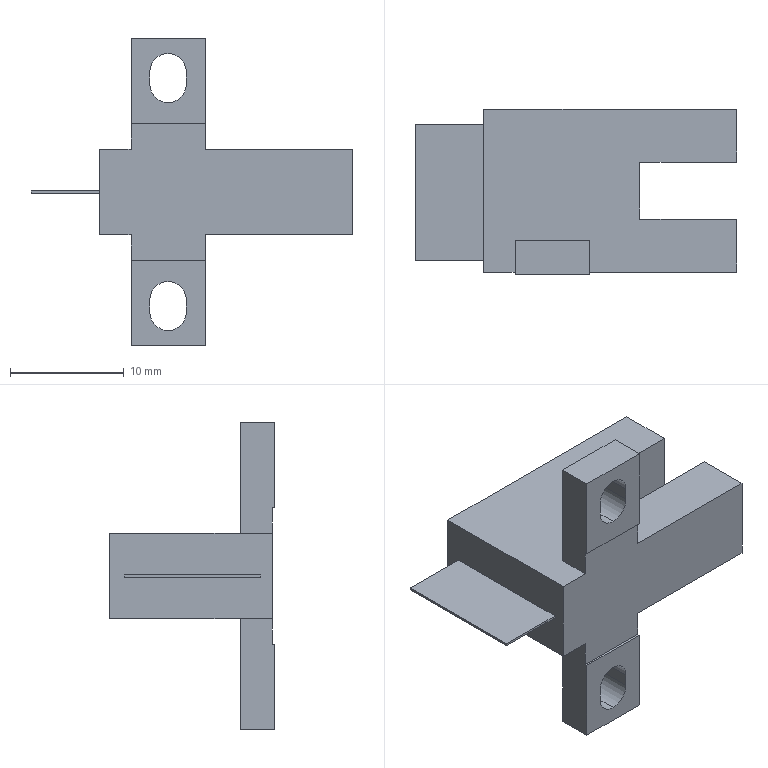Part | SolidWorks | features BaseBody 1 | 1 solid | 37 faces | box 28.2 x 14.5 x 27 mm | volume 2382 mm3 | plane 31 | cylinder 6 | commonest cylinder face diameters 3.2 x6
STEP:
#1=CARTESIAN_POINT('',(6.,2.8,7.85));
#2=VERTEX_POINT('',#1);
#3=CARTESIAN_POINT('',(7.6,2.8,9.45));
#4=VERTEX_POINT('',#3);
#5=CARTESIAN_POINT('',(6.,2.8,9.45));
#6=DIRECTION('',(0.,-1.,0.));
#7=DIRECTION('',(0.,0.,1.));
#8=AXIS2_PLACEMENT_3D('',#5,#6,#7);
#9=CIRCLE('',#8,1.6);
#10=EDGE_CURVE('',#2,#4,#9,.T.);
#11=ORIENTED_EDGE('',*,*,#10,.F.);
#12=CARTESIAN_POINT('',(6.,-0.2,7.85));
#13=VERTEX_POINT('',#12);
#14=CARTESIAN_POINT('',(6.,2.8,7.85));
#15=DIRECTION('',(0.,-1.,0.));
#16=VECTOR('',#15,1000.);
#17=LINE('',#14,#16);
#18=EDGE_CURVE('',#2,#13,#17,.T.);
#19=ORIENTED_EDGE('',*,*,#18,.T.);
#20=CARTESIAN_POINT('',(7.6,-0.2,9.45));
#21=VERTEX_POINT('',#20);
#22=CARTESIAN_POINT('',(6.,-0.2,9.45));
#23=DIRECTION('',(0.,-1.,0.));
#24=DIRECTION('',(0.,0.,1.));
#25=AXIS2_PLACEMENT_3D('',#22,#23,#24);
#26=CIRCLE('',#25,1.6);
#27=EDGE_CURVE('',#13,#21,#26,.T.);
#28=ORIENTED_EDGE('',*,*,#27,.T.);
#29=CARTESIAN_POINT('',(7.6,2.8,9.45));
#30=DIRECTION('',(0.,-1.,0.));
#31=VECTOR('',#30,1000.);
#32=LINE('',#29,#31);
#33=EDGE_CURVE('',#4,#21,#32,.T.);
#34=ORIENTED_EDGE('',*,*,#33,.F.);
#35=EDGE_LOOP('',(#11,#19,#28,#34));
#36=FACE_OUTER_BOUND('',#35,.T.);
#37=CARTESIAN_POINT('',(6.,2.8,9.45));
#38=DIRECTION('',(0.,-1.,0.));
#39=DIRECTION('',(0.,0.,-1.));
#40=AXIS2_PLACEMENT_3D('',#37,#38,#39);
#41=CYLINDRICAL_SURFACE('',#40,1.6);
#42=ADVANCED_FACE('',(#36),#41,.F.);
#43=CARTESIAN_POINT('',(6.,2.8,-12.15));
#44=VERTEX_POINT('',#43);
#45=CARTESIAN_POINT('',(7.6,2.8,-10.55));
#46=VERTEX_POINT('',#45);
#47=CARTESIAN_POINT('',(6.,2.8,-10.55));
#48=DIRECTION('',(0.,-1.,0.));
#49=DIRECTION('',(0.,0.,-1.));
#50=AXIS2_PLACEMENT_3D('',#47,#48,#49);
#51=CIRCLE('',#50,1.6);
#52=EDGE_CURVE('',#44,#46,#51,.T.);
#53=ORIENTED_EDGE('',*,*,#52,.F.);
#54=CARTESIAN_POINT('',(6.,-0.2,-12.15));
#55=VERTEX_POINT('',#54);
#56=CARTESIAN_POINT('',(6.,2.8,-12.15));
#57=DIRECTION('',(0.,-1.,0.));
#58=VECTOR('',#57,1000.);
#59=LINE('',#56,#58);
#60=EDGE_CURVE('',#44,#55,#59,.T.);
#61=ORIENTED_EDGE('',*,*,#60,.T.);
#62=CARTESIAN_POINT('',(7.6,-0.2,-10.55));
#63=VERTEX_POINT('',#62);
#64=CARTESIAN_POINT('',(6.,-0.2,-10.55));
#65=DIRECTION('',(0.,-1.,0.));
#66=DIRECTION('',(0.,0.,-1.));
#67=AXIS2_PLACEMENT_3D('',#64,#65,#66);
#68=CIRCLE('',#67,1.6);
#69=EDGE_CURVE('',#55,#63,#68,.T.);
#70=ORIENTED_EDGE('',*,*,#69,.T.);
#71=CARTESIAN_POINT('',(7.6,2.8,-10.55));
#72=DIRECTION('',(0.,-1.,0.));
#73=VECTOR('',#72,1000.);
#74=LINE('',#71,#73);
#75=EDGE_CURVE('',#46,#63,#74,.T.);
#76=ORIENTED_EDGE('',*,*,#75,.F.);
#77=EDGE_LOOP('',(#53,#61,#70,#76));
#78=FACE_OUTER_BOUND('',#77,.T.);
#79=CARTESIAN_POINT('',(6.,2.8,-10.55));
#80=DIRECTION('',(0.,-1.,0.));
#81=DIRECTION('',(0.,0.,-1.));
#82=AXIS2_PLACEMENT_3D('',#79,#80,#81);
#83=CYLINDRICAL_SURFACE('',#82,1.6);
#84=ADVANCED_FACE('',(#78),#83,.F.);
#85=CARTESIAN_POINT('',(-6.,13.,-0.1));
#86=VERTEX_POINT('',#85);
#87=CARTESIAN_POINT('',(-6.,1.,-0.1));
#88=VERTEX_POINT('',#87);
#89=CARTESIAN_POINT('',(-6.,13.,-0.1));
#90=DIRECTION('',(0.,-1.,0.));
#91=VECTOR('',#90,1000.);
#92=LINE('',#89,#91);
#93=EDGE_CURVE('',#86,#88,#92,.T.);
#94=ORIENTED_EDGE('',*,*,#93,.T.);
#95=CARTESIAN_POINT('',(-6.,1.,0.1));
#96=VERTEX_POINT('',#95);
#97=CARTESIAN_POINT('',(-6.,1.,-0.1));
#98=DIRECTION('',(0.,0.,1.));
#99=VECTOR('',#98,1000.);
#100=LINE('',#97,#99);
#101=EDGE_CURVE('',#88,#96,#100,.T.);
#102=ORIENTED_EDGE('',*,*,#101,.T.);
#103=CARTESIAN_POINT('',(-6.,13.,0.1));
#104=VERTEX_POINT('',#103);
#105=CARTESIAN_POINT('',(-6.,13.,0.1));
#106=DIRECTION('',(0.,1.,0.));
#107=VECTOR('',#106,1000.);
#108=LINE('',#105,#107);
#109=EDGE_CURVE('',#96,#104,#108,.T.);
#110=ORIENTED_EDGE('',*,*,#109,.T.);
#111=CARTESIAN_POINT('',(-6.,13.,-0.1));
#112=DIRECTION('',(0.,0.,-1.));
#113=VECTOR('',#112,1000.);
#114=LINE('',#111,#113);
#115=EDGE_CURVE('',#104,#86,#114,.T.);
#116=ORIENTED_EDGE('',*,*,#115,.T.);
#117=EDGE_LOOP('',(#94,#102,#110,#116));
#118=FACE_OUTER_BOUND('',#117,.T.);
#119=CARTESIAN_POINT('',(-6.,0.,0.));
#120=DIRECTION('',(-1.,0.,0.));
#121=DIRECTION('',(0.,0.,1.));
#122=AXIS2_PLACEMENT_3D('',#119,#120,#121);
#123=PLANE('',#122);
#124=ADVANCED_FACE('',(#118),#123,.T.);
#125=CARTESIAN_POINT('',(0.,13.,0.1));
#126=VERTEX_POINT('',#125);
#127=CARTESIAN_POINT('',(0.,13.,-0.1));
#128=VERTEX_POINT('',#127);
#129=CARTESIAN_POINT('',(0.,13.,-0.1));
#130=DIRECTION('',(0.,0.,-1.));
#131=VECTOR('',#130,1000.);
#132=LINE('',#129,#131);
#133=EDGE_CURVE('',#126,#128,#132,.T.);
#134=ORIENTED_EDGE('',*,*,#133,.T.);
#135=CARTESIAN_POINT('',(-6.,13.,-0.1));
#136=DIRECTION('',(1.,0.,0.));
#137=VECTOR('',#136,1000.);
#138=LINE('',#135,#137);
#139=EDGE_CURVE('',#86,#128,#138,.T.);
#140=ORIENTED_EDGE('',*,*,#139,.F.);
#141=ORIENTED_EDGE('',*,*,#115,.F.);
#142=CARTESIAN_POINT('',(-6.,13.,0.1));
#143=DIRECTION('',(1.,0.,0.));
#144=VECTOR('',#143,1000.);
#145=LINE('',#142,#144);
#146=EDGE_CURVE('',#104,#126,#145,.T.);
#147=ORIENTED_EDGE('',*,*,#146,.T.);
#148=EDGE_LOOP('',(#134,#140,#141,#147));
#149=FACE_OUTER_BOUND('',#148,.T.);
#150=CARTESIAN_POINT('',(-6.,13.,-0.1));
#151=DIRECTION('',(0.,-1.,0.));
#152=DIRECTION('',(-1.,0.,0.));
#153=AXIS2_PLACEMENT_3D('',#150,#151,#152);
#154=PLANE('',#153);
#155=ADVANCED_FACE('',(#149),#154,.F.);
#156=CARTESIAN_POINT('',(0.,1.,0.1));
#157=VERTEX_POINT('',#156);
#158=CARTESIAN_POINT('',(0.,13.,0.1));
#159=DIRECTION('',(0.,1.,0.));
#160=VECTOR('',#159,1000.);
#161=LINE('',#158,#160);
#162=EDGE_CURVE('',#157,#126,#161,.T.);
#163=ORIENTED_EDGE('',*,*,#162,.T.);
#164=ORIENTED_EDGE('',*,*,#146,.F.);
#165=ORIENTED_EDGE('',*,*,#109,.F.);
#166=CARTESIAN_POINT('',(-6.,1.,0.1));
#167=DIRECTION('',(1.,0.,0.));
#168=VECTOR('',#167,1000.);
#169=LINE('',#166,#168);
#170=EDGE_CURVE('',#96,#157,#169,.T.);
#171=ORIENTED_EDGE('',*,*,#170,.T.);
#172=EDGE_LOOP('',(#163,#164,#165,#171));
#173=FACE_OUTER_BOUND('',#172,.T.);
#174=CARTESIAN_POINT('',(-6.,13.,0.1));
#175=DIRECTION('',(0.,0.,-1.));
#176=DIRECTION('',(0.,-1.,0.));
#177=AXIS2_PLACEMENT_3D('',#174,#175,#176);
#178=PLANE('',#177);
#179=ADVANCED_FACE('',(#173),#178,.F.);
#180=CARTESIAN_POINT('',(0.,1.,-0.1));
#181=VERTEX_POINT('',#180);
#182=CARTESIAN_POINT('',(0.,1.,-0.1));
#183=DIRECTION('',(0.,0.,1.));
#184=VECTOR('',#183,1000.);
#185=LINE('',#182,#184);
#186=EDGE_CURVE('',#181,#157,#185,.T.);
#187=ORIENTED_EDGE('',*,*,#186,.T.);
#188=ORIENTED_EDGE('',*,*,#170,.F.);
#189=ORIENTED_EDGE('',*,*,#101,.F.);
#190=CARTESIAN_POINT('',(-6.,1.,-0.1));
#191=DIRECTION('',(1.,0.,0.));
#192=VECTOR('',#191,1000.);
#193=LINE('',#190,#192);
#194=EDGE_CURVE('',#88,#181,#193,.T.);
#195=ORIENTED_EDGE('',*,*,#194,.T.);
#196=EDGE_LOOP('',(#187,#188,#189,#195));
#197=FACE_OUTER_BOUND('',#196,.T.);
#198=CARTESIAN_POINT('',(-6.,1.,-0.1));
#199=DIRECTION('',(0.,1.,0.));
#200=DIRECTION('',(1.,0.,0.));
#201=AXIS2_PLACEMENT_3D('',#198,#199,#200);
#202=PLANE('',#201);
#203=ADVANCED_FACE('',(#197),#202,.F.);
#204=CARTESIAN_POINT('',(0.,13.,-0.1));
#205=DIRECTION('',(0.,-1.,0.));
#206=VECTOR('',#205,1000.);
#207=LINE('',#204,#206);
#208=EDGE_CURVE('',#128,#181,#207,.T.);
#209=ORIENTED_EDGE('',*,*,#208,.T.);
#210=ORIENTED_EDGE('',*,*,#194,.F.);
#211=ORIENTED_EDGE('',*,*,#93,.F.);
#212=ORIENTED_EDGE('',*,*,#139,.T.);
#213=EDGE_LOOP('',(#209,#210,#211,#212));
#214=FACE_OUTER_BOUND('',#213,.T.);
#215=CARTESIAN_POINT('',(-6.,13.,-0.1));
#216=DIRECTION('',(0.,0.,1.));
#217=DIRECTION('',(0.,-1.,0.));
#218=AXIS2_PLACEMENT_3D('',#215,#216,#217);
#219=PLANE('',#218);
#220=ADVANCED_FACE('',(#214),#219,.F.);
#221=CARTESIAN_POINT('',(9.25,-0.2,-6.));
#222=VERTEX_POINT('',#221);
#223=CARTESIAN_POINT('',(9.25,0.,-6.));
#224=VERTEX_POINT('',#223);
#225=CARTESIAN_POINT('',(9.25,-0.201,-6.));
#226=DIRECTION('',(0.,1.,0.));
#227=VECTOR('',#226,1000.);
#228=LINE('',#225,#227);
#229=EDGE_CURVE('',#222,#224,#228,.T.);
#230=ORIENTED_EDGE('',*,*,#229,.T.);
#231=CARTESIAN_POINT('',(2.75,0.,-6.));
#232=VERTEX_POINT('',#231);
#233=CARTESIAN_POINT('',(2.75,0.,-6.));
#234=DIRECTION('',(1.,0.,0.));
#235=VECTOR('',#234,1000.);
#236=LINE('',#233,#235);
#237=EDGE_CURVE('',#232,#224,#236,.T.);
#238=ORIENTED_EDGE('',*,*,#237,.F.);
#239=CARTESIAN_POINT('',(2.75,-0.2,-6.));
#240=VERTEX_POINT('',#239);
#241=CARTESIAN_POINT('',(2.75,-0.201,-6.));
#242=DIRECTION('',(0.,1.,0.));
#243=VECTOR('',#242,1000.);
#244=LINE('',#241,#243);
#245=EDGE_CURVE('',#240,#232,#244,.T.);
#246=ORIENTED_EDGE('',*,*,#245,.F.);
#247=CARTESIAN_POINT('',(2.75,-0.2,-6.));
#248=DIRECTION('',(-1.,0.,0.));
#249=VECTOR('',#248,1000.);
#250=LINE('',#247,#249);
#251=EDGE_CURVE('',#222,#240,#250,.T.);
#252=ORIENTED_EDGE('',*,*,#251,.F.);
#253=EDGE_LOOP('',(#230,#238,#246,#252));
#254=FACE_OUTER_BOUND('',#253,.T.);
#255=CARTESIAN_POINT('',(2.75,-0.201,-6.));
#256=DIRECTION('',(0.,0.,1.));
#257=DIRECTION('',(1.,0.,0.));
#258=AXIS2_PLACEMENT_3D('',#255,#256,#257);
#259=PLANE('',#258);
#260=ADVANCED_FACE('',(#254),#259,.T.);
#261=CARTESIAN_POINT('',(9.25,-0.2,6.));
#262=VERTEX_POINT('',#261);
#263=CARTESIAN_POINT('',(2.75,-0.2,6.));
#264=VERTEX_POINT('',#263);
#265=CARTESIAN_POINT('',(2.75,-0.2,6.));
#266=DIRECTION('',(-1.,0.,0.));
#267=VECTOR('',#266,1000.);
#268=LINE('',#265,#267);
#269=EDGE_CURVE('',#262,#264,#268,.T.);
#270=ORIENTED_EDGE('',*,*,#269,.T.);
#271=CARTESIAN_POINT('',(2.75,0.,6.));
#272=VERTEX_POINT('',#271);
#273=CARTESIAN_POINT('',(2.75,-0.201,6.));
#274=DIRECTION('',(0.,1.,0.));
#275=VECTOR('',#274,1000.);
#276=LINE('',#273,#275);
#277=EDGE_CURVE('',#264,#272,#276,.T.);
#278=ORIENTED_EDGE('',*,*,#277,.T.);
#279=CARTESIAN_POINT('',(9.25,0.,6.));
#280=VERTEX_POINT('',#279);
#281=CARTESIAN_POINT('',(2.75,0.,6.));
#282=DIRECTION('',(-1.,0.,0.));
#283=VECTOR('',#282,1000.);
#284=LINE('',#281,#283);
#285=EDGE_CURVE('',#280,#272,#284,.T.);
#286=ORIENTED_EDGE('',*,*,#285,.F.);
#287=CARTESIAN_POINT('',(9.25,-0.201,6.));
#288=DIRECTION('',(0.,1.,0.));
#289=VECTOR('',#288,1000.);
#290=LINE('',#287,#289);
#291=EDGE_CURVE('',#262,#280,#290,.T.);
#292=ORIENTED_EDGE('',*,*,#291,.F.);
#293=EDGE_LOOP('',(#270,#278,#286,#292));
#294=FACE_OUTER_BOUND('',#293,.T.);
#295=CARTESIAN_POINT('',(2.75,-0.201,6.));
#296=DIRECTION('',(0.,0.,-1.));
#297=DIRECTION('',(0.,-1.,0.));
#298=AXIS2_PLACEMENT_3D('',#295,#296,#297);
#299=PLANE('',#298);
#300=ADVANCED_FACE('',(#294),#299,.T.);
#301=CARTESIAN_POINT('',(4.4,2.8,10.55));
#302=VERTEX_POINT('',#301);
#303=CARTESIAN_POINT('',(4.4,-0.2,10.55));
#304=VERTEX_POINT('',#303);
#305=CARTESIAN_POINT('',(4.4,2.8,10.55));
#306=DIRECTION('',(0.,-1.,0.));
#307=VECTOR('',#306,1000.);
#308=LINE('',#305,#307);
#309=EDGE_CURVE('',#302,#304,#308,.T.);
#310=ORIENTED_EDGE('',*,*,#309,.T.);
#311=CARTESIAN_POINT('',(4.4,-0.2,9.45));
#312=VERTEX_POINT('',#311);
#313=CARTESIAN_POINT('',(4.4,-0.2,10.55));
#314=DIRECTION('',(0.,0.,-1.));
#315=VECTOR('',#314,1000.);
#316=LINE('',#313,#315);
#317=EDGE_CURVE('',#304,#312,#316,.T.);
#318=ORIENTED_EDGE('',*,*,#317,.T.);
#319=CARTESIAN_POINT('',(4.4,2.8,9.45));
#320=VERTEX_POINT('',#319);
#321=CARTESIAN_POINT('',(4.4,2.8,9.45));
#322=DIRECTION('',(0.,-1.,0.));
#323=VECTOR('',#322,1000.);
#324=LINE('',#321,#323);
#325=EDGE_CURVE('',#320,#312,#324,.T.);
#326=ORIENTED_EDGE('',*,*,#325,.F.);
#327=CARTESIAN_POINT('',(4.4,2.8,10.55));
#328=DIRECTION('',(0.,0.,-1.));
#329=VECTOR('',#328,1000.);
#330=LINE('',#327,#329);
#331=EDGE_CURVE('',#302,#320,#330,.T.);
#332=ORIENTED_EDGE('',*,*,#331,.F.);
#333=EDGE_LOOP('',(#310,#318,#326,#332));
#334=FACE_OUTER_BOUND('',#333,.T.);
#335=CARTESIAN_POINT('',(4.4,2.8,10.55));
#336=DIRECTION('',(-1.,0.,0.));
#337=DIRECTION('',(0.,0.,1.));
#338=AXIS2_PLACEMENT_3D('',#335,#336,#337);
#339=PLANE('',#338);
#340=ADVANCED_FACE('',(#334),#339,.F.);
#341=ORIENTED_EDGE('',*,*,#33,.T.);
#342=CARTESIAN_POINT('',(7.6,-0.2,10.55));
#343=VERTEX_POINT('',#342);
#344=CARTESIAN_POINT('',(7.6,-0.2,10.55));
#345=DIRECTION('',(0.,0.,1.));
#346=VECTOR('',#345,1000.);
#347=LINE('',#344,#346);
#348=EDGE_CURVE('',#21,#343,#347,.T.);
#349=ORIENTED_EDGE('',*,*,#348,.T.);
#350=CARTESIAN_POINT('',(7.6,2.8,10.55));
#351=VERTEX_POINT('',#350);
#352=CARTESIAN_POINT('',(7.6,2.8,10.55));
#353=DIRECTION('',(0.,-1.,0.));
#354=VECTOR('',#353,1000.);
#355=LINE('',#352,#354);
#356=EDGE_CURVE('',#351,#343,#355,.T.);
#357=ORIENTED_EDGE('',*,*,#356,.F.);
#358=CARTESIAN_POINT('',(7.6,2.8,10.55));
#359=DIRECTION('',(0.,0.,1.));
#360=VECTOR('',#359,1000.);
#361=LINE('',#358,#360);
#362=EDGE_CURVE('',#4,#351,#361,.T.);
#363=ORIENTED_EDGE('',*,*,#362,.F.);
#364=EDGE_LOOP('',(#341,#349,#357,#363));
#365=FACE_OUTER_BOUND('',#364,.T.);
#366=CARTESIAN_POINT('',(7.6,2.8,10.55));
#367=DIRECTION('',(1.,0.,0.));
#368=DIRECTION('',(0.,1.,0.));
#369=AXIS2_PLACEMENT_3D('',#366,#367,#368);
#370=PLANE('',#369);
#371=ADVANCED_FACE('',(#365),#370,.F.);
#372=ORIENTED_EDGE('',*,*,#356,.T.);
#373=CARTESIAN_POINT('',(6.,-0.2,10.55));
#374=DIRECTION('',(0.,-1.,0.));
#375=DIRECTION('',(0.,0.,1.));
#376=AXIS2_PLACEMENT_3D('',#373,#374,#375);
#377=CIRCLE('',#376,1.6);
#378=EDGE_CURVE('',#343,#304,#377,.T.);
#379=ORIENTED_EDGE('',*,*,#378,.T.);
#380=ORIENTED_EDGE('',*,*,#309,.F.);
#381=CARTESIAN_POINT('',(6.,2.8,10.55));
#382=DIRECTION('',(0.,-1.,0.));
#383=DIRECTION('',(0.,0.,1.));
#384=AXIS2_PLACEMENT_3D('',#381,#382,#383);
#385=CIRCLE('',#384,1.6);
#386=EDGE_CURVE('',#351,#302,#385,.T.);
#387=ORIENTED_EDGE('',*,*,#386,.F.);
#388=EDGE_LOOP('',(#372,#379,#380,#387));
#389=FACE_OUTER_BOUND('',#388,.T.);
#390=CARTESIAN_POINT('',(6.,2.8,10.55));
#391=DIRECTION('',(0.,-1.,0.));
#392=DIRECTION('',(0.,0.,-1.));
#393=AXIS2_PLACEMENT_3D('',#390,#391,#392);
#394=CYLINDRICAL_SURFACE('',#393,1.6);
#395=ADVANCED_FACE('',(#389),#394,.F.);
#396=ORIENTED_EDGE('',*,*,#362,.T.);
#397=ORIENTED_EDGE('',*,*,#386,.T.);
#398=ORIENTED_EDGE('',*,*,#331,.T.);
#399=CARTESIAN_POINT('',(6.,2.8,9.45));
#400=DIRECTION('',(0.,-1.,0.));
#401=DIRECTION('',(0.,0.,1.));
#402=AXIS2_PLACEMENT_3D('',#399,#400,#401);
#403=CIRCLE('',#402,1.6);
#404=EDGE_CURVE('',#320,#2,#403,.T.);
#405=ORIENTED_EDGE('',*,*,#404,.T.);
#406=ORIENTED_EDGE('',*,*,#10,.T.);
#407=EDGE_LOOP('',(#396,#397,#398,#405,#406));
#408=FACE_BOUND('',#407,.T.);
#409=CARTESIAN_POINT('',(9.25,2.8,3.75));
#410=VERTEX_POINT('',#409);
#411=CARTESIAN_POINT('',(9.25,2.8,13.5));
#412=VERTEX_POINT('',#411);
#413=CARTESIAN_POINT('',(9.25,2.8,3.75));
#414=DIRECTION('',(0.,0.,1.));
#415=VECTOR('',#414,1000.);
#416=LINE('',#413,#415);
#417=EDGE_CURVE('',#410,#412,#416,.T.);
#418=ORIENTED_EDGE('',*,*,#417,.F.);
#419=CARTESIAN_POINT('',(2.75,2.8,3.75));
#420=VERTEX_POINT('',#419);
#421=CARTESIAN_POINT('',(9.25,2.8,3.75));
#422=DIRECTION('',(1.,0.,0.));
#423=VECTOR('',#422,1000.);
#424=LINE('',#421,#423);
#425=EDGE_CURVE('',#420,#410,#424,.T.);
#426=ORIENTED_EDGE('',*,*,#425,.F.);
#427=CARTESIAN_POINT('',(2.75,2.8,13.5));
#428=VERTEX_POINT('',#427);
#429=CARTESIAN_POINT('',(2.75,2.8,3.75));
#430=DIRECTION('',(0.,0.,-1.));
#431=VECTOR('',#430,1000.);
#432=LINE('',#429,#431);
#433=EDGE_CURVE('',#428,#420,#432,.T.);
#434=ORIENTED_EDGE('',*,*,#433,.F.);
#435=CARTESIAN_POINT('',(9.25,2.8,13.5));
#436=DIRECTION('',(-1.,0.,0.));
#437=VECTOR('',#436,1000.);
#438=LINE('',#435,#437);
#439=EDGE_CURVE('',#412,#428,#438,.T.);
#440=ORIENTED_EDGE('',*,*,#439,.F.);
#441=EDGE_LOOP('',(#418,#426,#434,#440));
#442=FACE_OUTER_BOUND('',#441,.T.);
#443=CARTESIAN_POINT('',(0.,2.8,0.));
#444=DIRECTION('',(0.,-1.,0.));
#445=DIRECTION('',(0.,0.,-1.));
#446=AXIS2_PLACEMENT_3D('',#443,#444,#445);
#447=PLANE('',#446);
#448=ADVANCED_FACE('',(#408,#442),#447,.F.);
#449=CARTESIAN_POINT('',(2.75,-0.2,13.5));
#450=VERTEX_POINT('',#449);
#451=CARTESIAN_POINT('',(2.75,2.8,13.5));
#452=DIRECTION('',(0.,-1.,0.));
#453=VECTOR('',#452,1000.);
#454=LINE('',#451,#453);
#455=EDGE_CURVE('',#428,#450,#454,.T.);
#456=ORIENTED_EDGE('',*,*,#455,.T.);
#457=CARTESIAN_POINT('',(9.25,-0.2,13.5));
#458=VERTEX_POINT('',#457);
#459=CARTESIAN_POINT('',(9.25,-0.2,13.5));
#460=DIRECTION('',(-1.,0.,0.));
#461=VECTOR('',#460,1000.);
#462=LINE('',#459,#461);
#463=EDGE_CURVE('',#458,#450,#462,.T.);
#464=ORIENTED_EDGE('',*,*,#463,.F.);
#465=CARTESIAN_POINT('',(9.25,2.8,13.5));
#466=DIRECTION('',(0.,-1.,0.));
#467=VECTOR('',#466,1000.);
#468=LINE('',#465,#467);
#469=EDGE_CURVE('',#412,#458,#468,.T.);
#470=ORIENTED_EDGE('',*,*,#469,.F.);
#471=ORIENTED_EDGE('',*,*,#439,.T.);
#472=EDGE_LOOP('',(#456,#464,#470,#471));
#473=FACE_OUTER_BOUND('',#472,.T.);
#474=CARTESIAN_POINT('',(9.25,2.8,13.5));
#475=DIRECTION('',(0.,0.,1.));
#476=DIRECTION('',(1.,0.,0.));
#477=AXIS2_PLACEMENT_3D('',#474,#475,#476);
#478=PLANE('',#477);
#479=ADVANCED_FACE('',(#473),#478,.T.);
#480=CARTESIAN_POINT('',(2.75,0.,3.75));
#481=VERTEX_POINT('',#480);
#482=CARTESIAN_POINT('',(2.75,0.,-6.));
#483=DIRECTION('',(0.,0.,-1.));
#484=VECTOR('',#483,1000.);
#485=LINE('',#482,#484);
#486=EDGE_CURVE('',#272,#481,#485,.T.);
#487=ORIENTED_EDGE('',*,*,#486,.F.);
#488=ORIENTED_EDGE('',*,*,#277,.F.);
#489=CARTESIAN_POINT('',(2.75,-0.2,3.75));
#490=DIRECTION('',(0.,0.,-1.));
#491=VECTOR('',#490,1000.);
#492=LINE('',#489,#491);
#493=EDGE_CURVE('',#450,#264,#492,.T.);
#494=ORIENTED_EDGE('',*,*,#493,.F.);
#495=ORIENTED_EDGE('',*,*,#455,.F.);
#496=ORIENTED_EDGE('',*,*,#433,.T.);
#497=CARTESIAN_POINT('',(2.75,2.8,3.75));
#498=DIRECTION('',(0.,-1.,0.));
#499=VECTOR('',#498,1000.);
#500=LINE('',#497,#499);
#501=EDGE_CURVE('',#420,#481,#500,.T.);
#502=ORIENTED_EDGE('',*,*,#501,.T.);
#503=EDGE_LOOP('',(#487,#488,#494,#495,#496,#502));
#504=FACE_OUTER_BOUND('',#503,.T.);
#505=CARTESIAN_POINT('',(2.75,2.8,3.75));
#506=DIRECTION('',(-1.,0.,0.));
#507=DIRECTION('',(0.,1.,0.));
#508=AXIS2_PLACEMENT_3D('',#505,#506,#507);
#509=PLANE('',#508);
#510=ADVANCED_FACE('',(#504),#509,.T.);
#511=CARTESIAN_POINT('',(9.25,0.,3.75));
#512=VERTEX_POINT('',#511);
#513=CARTESIAN_POINT('',(9.25,0.,-6.));
#514=DIRECTION('',(0.,0.,1.));
#515=VECTOR('',#514,1000.);
#516=LINE('',#513,#515);
#517=EDGE_CURVE('',#512,#280,#516,.T.);
#518=ORIENTED_EDGE('',*,*,#517,.F.);
#519=CARTESIAN_POINT('',(9.25,2.8,3.75));
#520=DIRECTION('',(0.,-1.,0.));
#521=VECTOR('',#520,1000.);
#522=LINE('',#519,#521);
#523=EDGE_CURVE('',#410,#512,#522,.T.);
#524=ORIENTED_EDGE('',*,*,#523,.F.);
#525=ORIENTED_EDGE('',*,*,#417,.T.);
#526=ORIENTED_EDGE('',*,*,#469,.T.);
#527=CARTESIAN_POINT('',(9.25,-0.2,3.75));
#528=DIRECTION('',(0.,0.,1.));
#529=VECTOR('',#528,1000.);
#530=LINE('',#527,#529);
#531=EDGE_CURVE('',#262,#458,#530,.T.);
#532=ORIENTED_EDGE('',*,*,#531,.F.);
#533=ORIENTED_EDGE('',*,*,#291,.T.);
#534=EDGE_LOOP('',(#518,#524,#525,#526,#532,#533));
#535=FACE_OUTER_BOUND('',#534,.T.);
#536=CARTESIAN_POINT('',(9.25,2.8,3.75));
#537=DIRECTION('',(1.,0.,0.));
#538=DIRECTION('',(0.,0.,1.));
#539=AXIS2_PLACEMENT_3D('',#536,#537,#538);
#540=PLANE('',#539);
#541=ADVANCED_FACE('',(#535),#540,.T.);
#542=ORIENTED_EDGE('',*,*,#75,.T.);
#543=CARTESIAN_POINT('',(7.6,-0.2,-9.45));
#544=VERTEX_POINT('',#543);
#545=CARTESIAN_POINT('',(7.6,-0.2,-10.55));
#546=DIRECTION('',(0.,0.,1.));
#547=VECTOR('',#546,1000.);
#548=LINE('',#545,#547);
#549=EDGE_CURVE('',#63,#544,#548,.T.);
#550=ORIENTED_EDGE('',*,*,#549,.T.);
#551=CARTESIAN_POINT('',(7.6,2.8,-9.45));
#552=VERTEX_POINT('',#551);
#553=CARTESIAN_POINT('',(7.6,2.8,-9.45));
#554=DIRECTION('',(0.,-1.,0.));
#555=VECTOR('',#554,1000.);
#556=LINE('',#553,#555);
#557=EDGE_CURVE('',#552,#544,#556,.T.);
#558=ORIENTED_EDGE('',*,*,#557,.F.);
#559=CARTESIAN_POINT('',(7.6,2.8,-10.55));
#560=DIRECTION('',(0.,0.,1.));
#561=VECTOR('',#560,1000.);
#562=LINE('',#559,#561);
#563=EDGE_CURVE('',#46,#552,#562,.T.);
#564=ORIENTED_EDGE('',*,*,#563,.F.);
#565=EDGE_LOOP('',(#542,#550,#558,#564));
#566=FACE_OUTER_BOUND('',#565,.T.);
#567=CARTESIAN_POINT('',(7.6,2.8,-10.55));
#568=DIRECTION('',(1.,0.,0.));
#569=DIRECTION('',(0.,1.,0.));
#570=AXIS2_PLACEMENT_3D('',#567,#568,#569);
#571=PLANE('',#570);
#572=ADVANCED_FACE('',(#566),#571,.F.);
#573=ORIENTED_EDGE('',*,*,#557,.T.);
#574=CARTESIAN_POINT('',(4.4,-0.2,-9.45));
#575=VERTEX_POINT('',#574);
#576=CARTESIAN_POINT('',(6.,-0.2,-9.45));
#577=DIRECTION('',(0.,-1.,0.));
#578=DIRECTION('',(0.,0.,-1.));
#579=AXIS2_PLACEMENT_3D('',#576,#577,#578);
#580=CIRCLE('',#579,1.6);
#581=EDGE_CURVE('',#544,#575,#580,.T.);
#582=ORIENTED_EDGE('',*,*,#581,.T.);
#583=CARTESIAN_POINT('',(4.4,2.8,-9.45));
#584=VERTEX_POINT('',#583);
#585=CARTESIAN_POINT('',(4.4,2.8,-9.45));
#586=DIRECTION('',(0.,-1.,0.));
#587=VECTOR('',#586,1000.);
#588=LINE('',#585,#587);
#589=EDGE_CURVE('',#584,#575,#588,.T.);
#590=ORIENTED_EDGE('',*,*,#589,.F.);
#591=CARTESIAN_POINT('',(6.,2.8,-9.45));
#592=DIRECTION('',(0.,-1.,0.));
#593=DIRECTION('',(0.,0.,-1.));
#594=AXIS2_PLACEMENT_3D('',#591,#592,#593);
#595=CIRCLE('',#594,1.6);
#596=EDGE_CURVE('',#552,#584,#595,.T.);
#597=ORIENTED_EDGE('',*,*,#596,.F.);
#598=EDGE_LOOP('',(#573,#582,#590,#597));
#599=FACE_OUTER_BOUND('',#598,.T.);
#600=CARTESIAN_POINT('',(6.,2.8,-9.45));
#601=DIRECTION('',(0.,-1.,0.));
#602=DIRECTION('',(0.,0.,-1.));
#603=AXIS2_PLACEMENT_3D('',#600,#601,#602);
#604=CYLINDRICAL_SURFACE('',#603,1.6);
#605=ADVANCED_FACE('',(#599),#604,.F.);
#606=ORIENTED_EDGE('',*,*,#589,.T.);
#607=CARTESIAN_POINT('',(4.4,-0.2,-10.55));
#608=VERTEX_POINT('',#607);
#609=CARTESIAN_POINT('',(4.4,-0.2,-10.55));
#610=DIRECTION('',(0.,0.,-1.));
#611=VECTOR('',#610,1000.);
#612=LINE('',#609,#611);
#613=EDGE_CURVE('',#575,#608,#612,.T.);
#614=ORIENTED_EDGE('',*,*,#613,.T.);
#615=CARTESIAN_POINT('',(4.4,2.8,-10.55));
#616=VERTEX_POINT('',#615);
#617=CARTESIAN_POINT('',(4.4,2.8,-10.55));
#618=DIRECTION('',(0.,-1.,0.));
#619=VECTOR('',#618,1000.);
#620=LINE('',#617,#619);
#621=EDGE_CURVE('',#616,#608,#620,.T.);
#622=ORIENTED_EDGE('',*,*,#621,.F.);
#623=CARTESIAN_POINT('',(4.4,2.8,-10.55));
#624=DIRECTION('',(0.,0.,-1.));
#625=VECTOR('',#624,1000.);
#626=LINE('',#623,#625);
#627=EDGE_CURVE('',#584,#616,#626,.T.);
#628=ORIENTED_EDGE('',*,*,#627,.F.);
#629=EDGE_LOOP('',(#606,#614,#622,#628));
#630=FACE_OUTER_BOUND('',#629,.T.);
#631=CARTESIAN_POINT('',(4.4,2.8,-10.55));
#632=DIRECTION('',(-1.,0.,0.));
#633=DIRECTION('',(0.,0.,1.));
#634=AXIS2_PLACEMENT_3D('',#631,#632,#633);
#635=PLANE('',#634);
#636=ADVANCED_FACE('',(#630),#635,.F.);
#637=ORIENTED_EDGE('',*,*,#627,.T.);
#638=CARTESIAN_POINT('',(6.,2.8,-10.55));
#639=DIRECTION('',(0.,-1.,0.));
#640=DIRECTION('',(0.,0.,-1.));
#641=AXIS2_PLACEMENT_3D('',#638,#639,#640);
#642=CIRCLE('',#641,1.6);
#643=EDGE_CURVE('',#616,#44,#642,.T.);
#644=ORIENTED_EDGE('',*,*,#643,.T.);
#645=ORIENTED_EDGE('',*,*,#52,.T.);
#646=ORIENTED_EDGE('',*,*,#563,.T.);
#647=ORIENTED_EDGE('',*,*,#596,.T.);
#648=EDGE_LOOP('',(#637,#644,#645,#646,#647));
#649=FACE_BOUND('',#648,.T.);
#650=CARTESIAN_POINT('',(9.25,2.8,-13.5));
#651=VERTEX_POINT('',#650);
#652=CARTESIAN_POINT('',(9.25,2.8,-3.75));
#653=VERTEX_POINT('',#652);
#654=CARTESIAN_POINT('',(9.25,2.8,-3.75));
#655=DIRECTION('',(0.,0.,1.));
#656=VECTOR('',#655,1000.);
#657=LINE('',#654,#656);
#658=EDGE_CURVE('',#651,#653,#657,.T.);
#659=ORIENTED_EDGE('',*,*,#658,.F.);
#660=CARTESIAN_POINT('',(2.75,2.8,-13.5));
#661=VERTEX_POINT('',#660);
#662=CARTESIAN_POINT('',(9.25,2.8,-13.5));
#663=DIRECTION('',(1.,0.,0.));
#664=VECTOR('',#663,1000.);
#665=LINE('',#662,#664);
#666=EDGE_CURVE('',#661,#651,#665,.T.);
#667=ORIENTED_EDGE('',*,*,#666,.F.);
#668=CARTESIAN_POINT('',(2.75,2.8,-3.75));
#669=VERTEX_POINT('',#668);
#670=CARTESIAN_POINT('',(2.75,2.8,-3.75));
#671=DIRECTION('',(0.,0.,-1.));
#672=VECTOR('',#671,1000.);
#673=LINE('',#670,#672);
#674=EDGE_CURVE('',#669,#661,#673,.T.);
#675=ORIENTED_EDGE('',*,*,#674,.F.);
#676=CARTESIAN_POINT('',(9.25,2.8,-3.75));
#677=DIRECTION('',(-1.,0.,0.));
#678=VECTOR('',#677,1000.);
#679=LINE('',#676,#678);
#680=EDGE_CURVE('',#653,#669,#679,.T.);
#681=ORIENTED_EDGE('',*,*,#680,.F.);
#682=EDGE_LOOP('',(#659,#667,#675,#681));
#683=FACE_OUTER_BOUND('',#682,.T.);
#684=CARTESIAN_POINT('',(0.,2.8,0.));
#685=DIRECTION('',(0.,1.,0.));
#686=DIRECTION('',(1.,0.,0.));
#687=AXIS2_PLACEMENT_3D('',#684,#685,#686);
#688=PLANE('',#687);
#689=ADVANCED_FACE('',(#649,#683),#688,.T.);
#690=CARTESIAN_POINT('',(9.25,-0.2,-13.5));
#691=VERTEX_POINT('',#690);
#692=CARTESIAN_POINT('',(9.25,2.8,-13.5));
#693=DIRECTION('',(0.,-1.,0.));
#694=VECTOR('',#693,1000.);
#695=LINE('',#692,#694);
#696=EDGE_CURVE('',#651,#691,#695,.T.);
#697=ORIENTED_EDGE('',*,*,#696,.T.);
#698=CARTESIAN_POINT('',(2.75,-0.2,-13.5));
#699=VERTEX_POINT('',#698);
#700=CARTESIAN_POINT('',(9.25,-0.2,-13.5));
#701=DIRECTION('',(1.,0.,0.));
#702=VECTOR('',#701,1000.);
#703=LINE('',#700,#702);
#704=EDGE_CURVE('',#699,#691,#703,.T.);
#705=ORIENTED_EDGE('',*,*,#704,.F.);
#706=CARTESIAN_POINT('',(2.75,2.8,-13.5));
#707=DIRECTION('',(0.,-1.,0.));
#708=VECTOR('',#707,1000.);
#709=LINE('',#706,#708);
#710=EDGE_CURVE('',#661,#699,#709,.T.);
#711=ORIENTED_EDGE('',*,*,#710,.F.);
#712=ORIENTED_EDGE('',*,*,#666,.T.);
#713=EDGE_LOOP('',(#697,#705,#711,#712));
#714=FACE_OUTER_BOUND('',#713,.T.);
#715=CARTESIAN_POINT('',(9.25,2.8,-13.5));
#716=DIRECTION('',(0.,0.,-1.));
#717=DIRECTION('',(0.,-1.,0.));
#718=AXIS2_PLACEMENT_3D('',#715,#716,#717);
#719=PLANE('',#718);
#720=ADVANCED_FACE('',(#714),#719,.T.);
#721=ORIENTED_EDGE('',*,*,#680,.T.);
#722=CARTESIAN_POINT('',(2.75,0.,-3.75));
#723=VERTEX_POINT('',#722);
#724=CARTESIAN_POINT('',(2.75,2.8,-3.75));
#725=DIRECTION('',(0.,-1.,0.));
#726=VECTOR('',#725,1000.);
#727=LINE('',#724,#726);
#728=EDGE_CURVE('',#669,#723,#727,.T.);
#729=ORIENTED_EDGE('',*,*,#728,.T.);
#730=CARTESIAN_POINT('',(0.,0.,-3.75));
#731=VERTEX_POINT('',#730);
#732=CARTESIAN_POINT('',(0.,0.,-3.75));
#733=DIRECTION('',(1.,0.,0.));
#734=VECTOR('',#733,1000.);
#735=LINE('',#732,#734);
#736=EDGE_CURVE('',#731,#723,#735,.T.);
#737=ORIENTED_EDGE('',*,*,#736,.F.);
#738=CARTESIAN_POINT('',(0.,14.3,-3.75));
#739=VERTEX_POINT('',#738);
#740=CARTESIAN_POINT('',(0.,14.3,-3.75));
#741=DIRECTION('',(0.,-1.,0.));
#742=VECTOR('',#741,1000.);
#743=LINE('',#740,#742);
#744=EDGE_CURVE('',#739,#731,#743,.T.);
#745=ORIENTED_EDGE('',*,*,#744,.F.);
#746=CARTESIAN_POINT('',(22.2,14.3,-3.75));
#747=VERTEX_POINT('',#746);
#748=CARTESIAN_POINT('',(22.2,14.3,-3.75));
#749=DIRECTION('',(-1.,0.,0.));
#750=VECTOR('',#749,1000.);
#751=LINE('',#748,#750);
#752=EDGE_CURVE('',#747,#739,#751,.T.);
#753=ORIENTED_EDGE('',*,*,#752,.F.);
#754=CARTESIAN_POINT('',(22.2,9.65,-3.75));
#755=VERTEX_POINT('',#754);
#756=CARTESIAN_POINT('',(22.2,9.65,-3.75));
#757=DIRECTION('',(0.,1.,0.));
#758=VECTOR('',#757,1000.);
#759=LINE('',#756,#758);
#760=EDGE_CURVE('',#755,#747,#759,.T.);
#761=ORIENTED_EDGE('',*,*,#760,.F.);
#762=CARTESIAN_POINT('',(13.7,9.65,-3.75));
#763=VERTEX_POINT('',#762);
#764=CARTESIAN_POINT('',(13.7,9.65,-3.75));
#765=DIRECTION('',(1.,0.,0.));
#766=VECTOR('',#765,1000.);
#767=LINE('',#764,#766);
#768=EDGE_CURVE('',#763,#755,#767,.T.);
#769=ORIENTED_EDGE('',*,*,#768,.F.);
#770=CARTESIAN_POINT('',(13.7,4.65,-3.75));
#771=VERTEX_POINT('',#770);
#772=CARTESIAN_POINT('',(13.7,4.65,-3.75));
#773=DIRECTION('',(0.,1.,0.));
#774=VECTOR('',#773,1000.);
#775=LINE('',#772,#774);
#776=EDGE_CURVE('',#771,#763,#775,.T.);
#777=ORIENTED_EDGE('',*,*,#776,.F.);
#778=CARTESIAN_POINT('',(22.2,4.65,-3.75));
#779=VERTEX_POINT('',#778);
#780=CARTESIAN_POINT('',(22.2,4.65,-3.75));
#781=DIRECTION('',(-1.,0.,0.));
#782=VECTOR('',#781,1000.);
#783=LINE('',#780,#782);
#784=EDGE_CURVE('',#779,#771,#783,.T.);
#785=ORIENTED_EDGE('',*,*,#784,.F.);
#786=CARTESIAN_POINT('',(22.2,0.,-3.75));
#787=VERTEX_POINT('',#786);
#788=CARTESIAN_POINT('',(22.2,0.,-3.75));
#789=DIRECTION('',(0.,1.,0.));
#790=VECTOR('',#789,1000.);
#791=LINE('',#788,#790);
#792=EDGE_CURVE('',#787,#779,#791,.T.);
#793=ORIENTED_EDGE('',*,*,#792,.F.);
#794=CARTESIAN_POINT('',(9.25,0.,-3.75));
#795=VERTEX_POINT('',#794);
#796=CARTESIAN_POINT('',(0.,0.,-3.75));
#797=DIRECTION('',(1.,0.,0.));
#798=VECTOR('',#797,1000.);
#799=LINE('',#796,#798);
#800=EDGE_CURVE('',#795,#787,#799,.T.);
#801=ORIENTED_EDGE('',*,*,#800,.F.);
#802=CARTESIAN_POINT('',(9.25,2.8,-3.75));
#803=DIRECTION('',(0.,-1.,0.));
#804=VECTOR('',#803,1000.);
#805=LINE('',#802,#804);
#806=EDGE_CURVE('',#653,#795,#805,.T.);
#807=ORIENTED_EDGE('',*,*,#806,.F.);
#808=EDGE_LOOP('',(#721,#729,#737,#745,#753,#761,#769,#777,#785,#793,#801,#807));
#809=FACE_OUTER_BOUND('',#808,.T.);
#810=CARTESIAN_POINT('',(0.,0.,-3.75));
#811=DIRECTION('',(0.,0.,1.));
#812=DIRECTION('',(1.,0.,0.));
#813=AXIS2_PLACEMENT_3D('',#810,#811,#812);
#814=PLANE('',#813);
#815=ADVANCED_FACE('',(#809),#814,.F.);
#816=ORIENTED_EDGE('',*,*,#752,.T.);
#817=CARTESIAN_POINT('',(0.,14.3,3.75));
#818=VERTEX_POINT('',#817);
#819=CARTESIAN_POINT('',(0.,14.3,3.75));
#820=DIRECTION('',(0.,0.,-1.));
#821=VECTOR('',#820,1000.);
#822=LINE('',#819,#821);
#823=EDGE_CURVE('',#818,#739,#822,.T.);
#824=ORIENTED_EDGE('',*,*,#823,.F.);
#825=CARTESIAN_POINT('',(22.2,14.3,3.75));
#826=VERTEX_POINT('',#825);
#827=CARTESIAN_POINT('',(22.2,14.3,3.75));
#828=DIRECTION('',(-1.,0.,0.));
#829=VECTOR('',#828,1000.);
#830=LINE('',#827,#829);
#831=EDGE_CURVE('',#826,#818,#830,.T.);
#832=ORIENTED_EDGE('',*,*,#831,.F.);
#833=CARTESIAN_POINT('',(22.2,14.3,3.75));
#834=DIRECTION('',(0.,0.,-1.));
#835=VECTOR('',#834,1000.);
#836=LINE('',#833,#835);
#837=EDGE_CURVE('',#826,#747,#836,.T.);
#838=ORIENTED_EDGE('',*,*,#837,.T.);
#839=EDGE_LOOP('',(#816,#824,#832,#838));
#840=FACE_OUTER_BOUND('',#839,.T.);
#841=CARTESIAN_POINT('',(22.2,14.3,3.75));
#842=DIRECTION('',(0.,-1.,0.));
#843=DIRECTION('',(0.,0.,-1.));
#844=AXIS2_PLACEMENT_3D('',#841,#842,#843);
#845=PLANE('',#844);
#846=ADVANCED_FACE('',(#840),#845,.F.);
#847=ORIENTED_EDGE('',*,*,#760,.T.);
#848=ORIENTED_EDGE('',*,*,#837,.F.);
#849=CARTESIAN_POINT('',(22.2,9.65,3.75));
#850=VERTEX_POINT('',#849);
#851=CARTESIAN_POINT('',(22.2,9.65,3.75));
#852=DIRECTION('',(0.,1.,0.));
#853=VECTOR('',#852,1000.);
#854=LINE('',#851,#853);
#855=EDGE_CURVE('',#850,#826,#854,.T.);
#856=ORIENTED_EDGE('',*,*,#855,.F.);
#857=CARTESIAN_POINT('',(22.2,9.65,3.75));
#858=DIRECTION('',(0.,0.,-1.));
#859=VECTOR('',#858,1000.);
#860=LINE('',#857,#859);
#861=EDGE_CURVE('',#850,#755,#860,.T.);
#862=ORIENTED_EDGE('',*,*,#861,.T.);
#863=EDGE_LOOP('',(#847,#848,#856,#862));
#864=FACE_OUTER_BOUND('',#863,.T.);
#865=CARTESIAN_POINT('',(22.2,9.65,3.75));
#866=DIRECTION('',(-1.,0.,0.));
#867=DIRECTION('',(0.,0.,1.));
#868=AXIS2_PLACEMENT_3D('',#865,#866,#867);
#869=PLANE('',#868);
#870=ADVANCED_FACE('',(#864),#869,.F.);
#871=ORIENTED_EDGE('',*,*,#768,.T.);
#872=ORIENTED_EDGE('',*,*,#861,.F.);
#873=CARTESIAN_POINT('',(13.7,9.65,3.75));
#874=VERTEX_POINT('',#873);
#875=CARTESIAN_POINT('',(13.7,9.65,3.75));
#876=DIRECTION('',(1.,0.,0.));
#877=VECTOR('',#876,1000.);
#878=LINE('',#875,#877);
#879=EDGE_CURVE('',#874,#850,#878,.T.);
#880=ORIENTED_EDGE('',*,*,#879,.F.);
#881=CARTESIAN_POINT('',(13.7,9.65,3.75));
#882=DIRECTION('',(0.,0.,-1.));
#883=VECTOR('',#882,1000.);
#884=LINE('',#881,#883);
#885=EDGE_CURVE('',#874,#763,#884,.T.);
#886=ORIENTED_EDGE('',*,*,#885,.T.);
#887=EDGE_LOOP('',(#871,#872,#880,#886));
#888=FACE_OUTER_BOUND('',#887,.T.);
#889=CARTESIAN_POINT('',(13.7,9.65,3.75));
#890=DIRECTION('',(0.,1.,0.));
#891=DIRECTION('',(1.,0.,0.));
#892=AXIS2_PLACEMENT_3D('',#889,#890,#891);
#893=PLANE('',#892);
#894=ADVANCED_FACE('',(#888),#893,.F.);
#895=ORIENTED_EDGE('',*,*,#776,.T.);
#896=ORIENTED_EDGE('',*,*,#885,.F.);
#897=CARTESIAN_POINT('',(13.7,4.65,3.75));
#898=VERTEX_POINT('',#897);
#899=CARTESIAN_POINT('',(13.7,4.65,3.75));
#900=DIRECTION('',(0.,1.,0.));
#901=VECTOR('',#900,1000.);
#902=LINE('',#899,#901);
#903=EDGE_CURVE('',#898,#874,#902,.T.);
#904=ORIENTED_EDGE('',*,*,#903,.F.);
#905=CARTESIAN_POINT('',(13.7,4.65,3.75));
#906=DIRECTION('',(0.,0.,-1.));
#907=VECTOR('',#906,1000.);
#908=LINE('',#905,#907);
#909=EDGE_CURVE('',#898,#771,#908,.T.);
#910=ORIENTED_EDGE('',*,*,#909,.T.);
#911=EDGE_LOOP('',(#895,#896,#904,#910));
#912=FACE_OUTER_BOUND('',#911,.T.);
#913=CARTESIAN_POINT('',(13.7,4.65,3.75));
#914=DIRECTION('',(-1.,0.,0.));
#915=DIRECTION('',(0.,0.,1.));
#916=AXIS2_PLACEMENT_3D('',#913,#914,#915);
#917=PLANE('',#916);
#918=ADVANCED_FACE('',(#912),#917,.F.);
#919=ORIENTED_EDGE('',*,*,#784,.T.);
#920=ORIENTED_EDGE('',*,*,#909,.F.);
#921=CARTESIAN_POINT('',(22.2,4.65,3.75));
#922=VERTEX_POINT('',#921);
#923=CARTESIAN_POINT('',(22.2,4.65,3.75));
#924=DIRECTION('',(-1.,0.,0.));
#925=VECTOR('',#924,1000.);
#926=LINE('',#923,#925);
#927=EDGE_CURVE('',#922,#898,#926,.T.);
#928=ORIENTED_EDGE('',*,*,#927,.F.);
#929=CARTESIAN_POINT('',(22.2,4.65,3.75));
#930=DIRECTION('',(0.,0.,-1.));
#931=VECTOR('',#930,1000.);
#932=LINE('',#929,#931);
#933=EDGE_CURVE('',#922,#779,#932,.T.);
#934=ORIENTED_EDGE('',*,*,#933,.T.);
#935=EDGE_LOOP('',(#919,#920,#928,#934));
#936=FACE_OUTER_BOUND('',#935,.T.);
#937=CARTESIAN_POINT('',(22.2,4.65,3.75));
#938=DIRECTION('',(0.,-1.,0.));
#939=DIRECTION('',(0.,0.,-1.));
#940=AXIS2_PLACEMENT_3D('',#937,#938,#939);
#941=PLANE('',#940);
#942=ADVANCED_FACE('',(#936),#941,.F.);
#943=ORIENTED_EDGE('',*,*,#792,.T.);
#944=ORIENTED_EDGE('',*,*,#933,.F.);
#945=CARTESIAN_POINT('',(22.2,0.,3.75));
#946=VERTEX_POINT('',#945);
#947=CARTESIAN_POINT('',(22.2,0.,3.75));
#948=DIRECTION('',(0.,1.,0.));
#949=VECTOR('',#948,1000.);
#950=LINE('',#947,#949);
#951=EDGE_CURVE('',#946,#922,#950,.T.);
#952=ORIENTED_EDGE('',*,*,#951,.F.);
#953=CARTESIAN_POINT('',(22.2,0.,3.75));
#954=DIRECTION('',(0.,0.,-1.));
#955=VECTOR('',#954,1000.);
#956=LINE('',#953,#955);
#957=EDGE_CURVE('',#946,#787,#956,.T.);
#958=ORIENTED_EDGE('',*,*,#957,.T.);
#959=EDGE_LOOP('',(#943,#944,#952,#958));
#960=FACE_OUTER_BOUND('',#959,.T.);
#961=CARTESIAN_POINT('',(22.2,0.,3.75));
#962=DIRECTION('',(-1.,0.,0.));
#963=DIRECTION('',(0.,0.,1.));
#964=AXIS2_PLACEMENT_3D('',#961,#962,#963);
#965=PLANE('',#964);
#966=ADVANCED_FACE('',(#960),#965,.F.);
#967=ORIENTED_EDGE('',*,*,#736,.T.);
#968=CARTESIAN_POINT('',(2.75,0.,-6.));
#969=DIRECTION('',(0.,0.,-1.));
#970=VECTOR('',#969,1000.);
#971=LINE('',#968,#970);
#972=EDGE_CURVE('',#723,#232,#971,.T.);
#973=ORIENTED_EDGE('',*,*,#972,.T.);
#974=ORIENTED_EDGE('',*,*,#237,.T.);
#975=CARTESIAN_POINT('',(9.25,0.,-6.));
#976=DIRECTION('',(0.,0.,1.));
#977=VECTOR('',#976,1000.);
#978=LINE('',#975,#977);
#979=EDGE_CURVE('',#224,#795,#978,.T.);
#980=ORIENTED_EDGE('',*,*,#979,.T.);
#981=ORIENTED_EDGE('',*,*,#800,.T.);
#982=ORIENTED_EDGE('',*,*,#957,.F.);
#983=CARTESIAN_POINT('',(0.,0.,3.75));
#984=DIRECTION('',(1.,0.,0.));
#985=VECTOR('',#984,1000.);
#986=LINE('',#983,#985);
#987=EDGE_CURVE('',#512,#946,#986,.T.);
#988=ORIENTED_EDGE('',*,*,#987,.F.);
#989=ORIENTED_EDGE('',*,*,#517,.T.);
#990=ORIENTED_EDGE('',*,*,#285,.T.);
#991=ORIENTED_EDGE('',*,*,#486,.T.);
#992=CARTESIAN_POINT('',(0.,0.,3.75));
#993=VERTEX_POINT('',#992);
#994=CARTESIAN_POINT('',(0.,0.,3.75));
#995=DIRECTION('',(1.,0.,0.));
#996=VECTOR('',#995,1000.);
#997=LINE('',#994,#996);
#998=EDGE_CURVE('',#993,#481,#997,.T.);
#999=ORIENTED_EDGE('',*,*,#998,.F.);
#1000=CARTESIAN_POINT('',(0.,0.,3.75));
#1001=DIRECTION('',(0.,0.,-1.));
#1002=VECTOR('',#1001,1000.);
#1003=LINE('',#1000,#1002);
#1004=EDGE_CURVE('',#993,#731,#1003,.T.);
#1005=ORIENTED_EDGE('',*,*,#1004,.T.);
#1006=EDGE_LOOP('',(#967,#973,#974,#980,#981,#982,#988,#989,#990,#991,#999,#1005));
#1007=FACE_OUTER_BOUND('',#1006,.T.);
#1008=CARTESIAN_POINT('',(0.,0.,3.75));
#1009=DIRECTION('',(0.,1.,0.));
#1010=DIRECTION('',(1.,0.,0.));
#1011=AXIS2_PLACEMENT_3D('',#1008,#1009,#1010);
#1012=PLANE('',#1011);
#1013=ADVANCED_FACE('',(#1007),#1012,.F.);
#1014=ORIENTED_EDGE('',*,*,#425,.T.);
#1015=ORIENTED_EDGE('',*,*,#523,.T.);
#1016=ORIENTED_EDGE('',*,*,#987,.T.);
#1017=ORIENTED_EDGE('',*,*,#951,.T.);
#1018=ORIENTED_EDGE('',*,*,#927,.T.);
#1019=ORIENTED_EDGE('',*,*,#903,.T.);
#1020=ORIENTED_EDGE('',*,*,#879,.T.);
#1021=ORIENTED_EDGE('',*,*,#855,.T.);
#1022=ORIENTED_EDGE('',*,*,#831,.T.);
#1023=CARTESIAN_POINT('',(0.,14.3,3.75));
#1024=DIRECTION('',(0.,-1.,0.));
#1025=VECTOR('',#1024,1000.);
#1026=LINE('',#1023,#1025);
#1027=EDGE_CURVE('',#818,#993,#1026,.T.);
#1028=ORIENTED_EDGE('',*,*,#1027,.T.);
#1029=ORIENTED_EDGE('',*,*,#998,.T.);
#1030=ORIENTED_EDGE('',*,*,#501,.F.);
#1031=EDGE_LOOP('',(#1014,#1015,#1016,#1017,#1018,#1019,#1020,#1021,#1022,#1028,#1029,#1030));
#1032=FACE_OUTER_BOUND('',#1031,.T.);
#1033=CARTESIAN_POINT('',(0.,0.,3.75));
#1034=DIRECTION('',(0.,0.,1.));
#1035=DIRECTION('',(1.,0.,0.));
#1036=AXIS2_PLACEMENT_3D('',#1033,#1034,#1035);
#1037=PLANE('',#1036);
#1038=ADVANCED_FACE('',(#1032),#1037,.T.);
#1039=ORIENTED_EDGE('',*,*,#317,.F.);
#1040=ORIENTED_EDGE('',*,*,#378,.F.);
#1041=ORIENTED_EDGE('',*,*,#348,.F.);
#1042=ORIENTED_EDGE('',*,*,#27,.F.);
#1043=CARTESIAN_POINT('',(6.,-0.2,9.45));
#1044=DIRECTION('',(0.,-1.,0.));
#1045=DIRECTION('',(0.,0.,1.));
#1046=AXIS2_PLACEMENT_3D('',#1043,#1044,#1045);
#1047=CIRCLE('',#1046,1.6);
#1048=EDGE_CURVE('',#312,#13,#1047,.T.);
#1049=ORIENTED_EDGE('',*,*,#1048,.F.);
#1050=EDGE_LOOP('',(#1039,#1040,#1041,#1042,#1049));
#1051=FACE_BOUND('',#1050,.T.);
#1052=ORIENTED_EDGE('',*,*,#493,.T.);
#1053=ORIENTED_EDGE('',*,*,#269,.F.);
#1054=ORIENTED_EDGE('',*,*,#531,.T.);
#1055=ORIENTED_EDGE('',*,*,#463,.T.);
#1056=EDGE_LOOP('',(#1052,#1053,#1054,#1055));
#1057=FACE_OUTER_BOUND('',#1056,.T.);
#1058=CARTESIAN_POINT('',(0.,-0.2,0.));
#1059=DIRECTION('',(0.,-1.,0.));
#1060=DIRECTION('',(0.,0.,-1.));
#1061=AXIS2_PLACEMENT_3D('',#1058,#1059,#1060);
#1062=PLANE('',#1061);
#1063=ADVANCED_FACE('',(#1051,#1057),#1062,.T.);
#1064=CARTESIAN_POINT('',(6.,-0.2,-10.55));
#1065=DIRECTION('',(0.,-1.,0.));
#1066=DIRECTION('',(0.,0.,-1.));
#1067=AXIS2_PLACEMENT_3D('',#1064,#1065,#1066);
#1068=CIRCLE('',#1067,1.6);
#1069=EDGE_CURVE('',#608,#55,#1068,.T.);
#1070=ORIENTED_EDGE('',*,*,#1069,.F.);
#1071=ORIENTED_EDGE('',*,*,#613,.F.);
#1072=ORIENTED_EDGE('',*,*,#581,.F.);
#1073=ORIENTED_EDGE('',*,*,#549,.F.);
#1074=ORIENTED_EDGE('',*,*,#69,.F.);
#1075=EDGE_LOOP('',(#1070,#1071,#1072,#1073,#1074));
#1076=FACE_BOUND('',#1075,.T.);
#1077=ORIENTED_EDGE('',*,*,#251,.T.);
#1078=CARTESIAN_POINT('',(2.75,-0.2,-3.75));
#1079=DIRECTION('',(0.,0.,-1.));
#1080=VECTOR('',#1079,1000.);
#1081=LINE('',#1078,#1080);
#1082=EDGE_CURVE('',#240,#699,#1081,.T.);
#1083=ORIENTED_EDGE('',*,*,#1082,.T.);
#1084=ORIENTED_EDGE('',*,*,#704,.T.);
#1085=CARTESIAN_POINT('',(9.25,-0.2,-3.75));
#1086=DIRECTION('',(0.,0.,1.));
#1087=VECTOR('',#1086,1000.);
#1088=LINE('',#1085,#1087);
#1089=EDGE_CURVE('',#691,#222,#1088,.T.);
#1090=ORIENTED_EDGE('',*,*,#1089,.T.);
#1091=EDGE_LOOP('',(#1077,#1083,#1084,#1090));
#1092=FACE_OUTER_BOUND('',#1091,.T.);
#1093=CARTESIAN_POINT('',(0.,-0.2,0.));
#1094=DIRECTION('',(0.,1.,0.));
#1095=DIRECTION('',(1.,0.,0.));
#1096=AXIS2_PLACEMENT_3D('',#1093,#1094,#1095);
#1097=PLANE('',#1096);
#1098=ADVANCED_FACE('',(#1076,#1092),#1097,.F.);
#1099=ORIENTED_EDGE('',*,*,#1082,.F.);
#1100=ORIENTED_EDGE('',*,*,#245,.T.);
#1101=ORIENTED_EDGE('',*,*,#972,.F.);
#1102=ORIENTED_EDGE('',*,*,#728,.F.);
#1103=ORIENTED_EDGE('',*,*,#674,.T.);
#1104=ORIENTED_EDGE('',*,*,#710,.T.);
#1105=EDGE_LOOP('',(#1099,#1100,#1101,#1102,#1103,#1104));
#1106=FACE_OUTER_BOUND('',#1105,.T.);
#1107=CARTESIAN_POINT('',(2.75,2.8,-3.75));
#1108=DIRECTION('',(-1.,0.,0.));
#1109=DIRECTION('',(0.,0.,1.));
#1110=AXIS2_PLACEMENT_3D('',#1107,#1108,#1109);
#1111=PLANE('',#1110);
#1112=ADVANCED_FACE('',(#1106),#1111,.T.);
#1113=ORIENTED_EDGE('',*,*,#979,.F.);
#1114=ORIENTED_EDGE('',*,*,#229,.F.);
#1115=ORIENTED_EDGE('',*,*,#1089,.F.);
#1116=ORIENTED_EDGE('',*,*,#696,.F.);
#1117=ORIENTED_EDGE('',*,*,#658,.T.);
#1118=ORIENTED_EDGE('',*,*,#806,.T.);
#1119=EDGE_LOOP('',(#1113,#1114,#1115,#1116,#1117,#1118));
#1120=FACE_OUTER_BOUND('',#1119,.T.);
#1121=CARTESIAN_POINT('',(9.25,2.8,-3.75));
#1122=DIRECTION('',(1.,0.,0.));
#1123=DIRECTION('',(0.,0.,-1.));
#1124=AXIS2_PLACEMENT_3D('',#1121,#1122,#1123);
#1125=PLANE('',#1124);
#1126=ADVANCED_FACE('',(#1120),#1125,.T.);
#1127=ORIENTED_EDGE('',*,*,#208,.F.);
#1128=ORIENTED_EDGE('',*,*,#133,.F.);
#1129=ORIENTED_EDGE('',*,*,#162,.F.);
#1130=ORIENTED_EDGE('',*,*,#186,.F.);
#1131=EDGE_LOOP('',(#1127,#1128,#1129,#1130));
#1132=FACE_BOUND('',#1131,.T.);
#1133=ORIENTED_EDGE('',*,*,#744,.T.);
#1134=ORIENTED_EDGE('',*,*,#1004,.F.);
#1135=ORIENTED_EDGE('',*,*,#1027,.F.);
#1136=ORIENTED_EDGE('',*,*,#823,.T.);
#1137=EDGE_LOOP('',(#1133,#1134,#1135,#1136));
#1138=FACE_OUTER_BOUND('',#1137,.T.);
#1139=CARTESIAN_POINT('',(0.,14.3,3.75));
#1140=DIRECTION('',(1.,0.,0.));
#1141=DIRECTION('',(0.,-1.,0.));
#1142=AXIS2_PLACEMENT_3D('',#1139,#1140,#1141);
#1143=PLANE('',#1142);
#1144=ADVANCED_FACE('',(#1132,#1138),#1143,.F.);
#1145=ORIENTED_EDGE('',*,*,#60,.F.);
#1146=ORIENTED_EDGE('',*,*,#643,.F.);
#1147=ORIENTED_EDGE('',*,*,#621,.T.);
#1148=ORIENTED_EDGE('',*,*,#1069,.T.);
#1149=EDGE_LOOP('',(#1145,#1146,#1147,#1148));
#1150=FACE_OUTER_BOUND('',#1149,.T.);
#1151=CARTESIAN_POINT('',(6.,2.8,-10.55));
#1152=DIRECTION('',(0.,-1.,0.));
#1153=DIRECTION('',(0.,0.,-1.));
#1154=AXIS2_PLACEMENT_3D('',#1151,#1152,#1153);
#1155=CYLINDRICAL_SURFACE('',#1154,1.6);
#1156=ADVANCED_FACE('',(#1150),#1155,.F.);
#1157=ORIENTED_EDGE('',*,*,#18,.F.);
#1158=ORIENTED_EDGE('',*,*,#404,.F.);
#1159=ORIENTED_EDGE('',*,*,#325,.T.);
#1160=ORIENTED_EDGE('',*,*,#1048,.T.);
#1161=EDGE_LOOP('',(#1157,#1158,#1159,#1160));
#1162=FACE_OUTER_BOUND('',#1161,.T.);
#1163=CARTESIAN_POINT('',(6.,2.8,9.45));
#1164=DIRECTION('',(0.,-1.,0.));
#1165=DIRECTION('',(0.,0.,-1.));
#1166=AXIS2_PLACEMENT_3D('',#1163,#1164,#1165);
#1167=CYLINDRICAL_SURFACE('',#1166,1.6);
#1168=ADVANCED_FACE('',(#1162),#1167,.F.);
#1169=CLOSED_SHELL('',(#42,#84,#124,#155,#179,#203,#220,#260,#300,#340,#371,#395,#448,#479,#510,#541,#572,#605,#636,#689,#720,#815,#846,#870,#894,#918,#942,#966,#1013,#1038,#1063,#1098,#1112,#1126,#1144,#1156,#1168));
#1170=MANIFOLD_SOLID_BREP('',#1169);
#1171=CARTESIAN_POINT('',(0.,0.,0.));
#1172=DIRECTION('',(0.,0.,1.));
#1173=DIRECTION('',(1.,0.,0.));
#1174=AXIS2_PLACEMENT_3D('',#1171,#1172,#1173);
#1175=(LENGTH_UNIT()NAMED_UNIT(*)SI_UNIT(.MILLI.,.METRE.));
#1176=UNCERTAINTY_MEASURE_WITH_UNIT(LENGTH_MEASURE(0.00001),#1175,'','');
#1177=(NAMED_UNIT(*)PLANE_ANGLE_UNIT()SI_UNIT($,.RADIAN.));
#1178=(NAMED_UNIT(*)SI_UNIT($,.STERADIAN.)SOLID_ANGLE_UNIT());
#1179=(GEOMETRIC_REPRESENTATION_CONTEXT(3)GLOBAL_UNCERTAINTY_ASSIGNED_CONTEXT((#1176))GLOBAL_UNIT_ASSIGNED_CONTEXT((#1175,#1177,#1178))REPRESENTATION_CONTEXT('',''));
#1180=ADVANCED_BREP_SHAPE_REPRESENTATION('',(#1170,#1174),#1179);